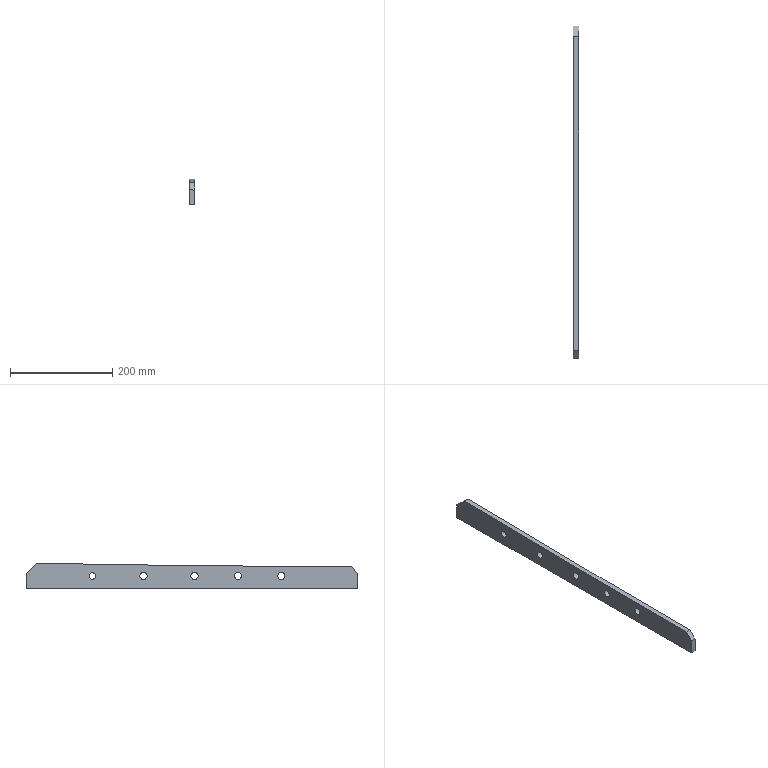Part | NX | features solid 2 | 1 solid | 13 faces | box 10 x 650.034 x 49.781 mm | volume 286400 mm3 | plane 5 | cylinder 5 | spline 3 | commonest cylinder face diameters 14 x4 13 x1
STEP:
#1=CARTESIAN_POINT('',(65.,-179.966,-104.));
#2=VERTEX_POINT('',#1);
#3=CARTESIAN_POINT('',(65.,-179.966,-97.));
#4=DIRECTION('',(1.,0.,0.));
#5=DIRECTION('',(0.,0.,-1.));
#6=AXIS2_PLACEMENT_3D('',#3,#4,#5);
#7=CIRCLE('',#6,7.);
#8=EDGE_CURVE('',#2,#2,#7,.F.);
#9=ORIENTED_EDGE('',*,*,#8,.T.);
#10=EDGE_LOOP('',(#9));
#11=FACE_BOUND('',#10,.T.);
#12=CARTESIAN_POINT('',(65.,-9.966,-104.));
#13=VERTEX_POINT('',#12);
#14=CARTESIAN_POINT('',(65.,-9.966,-97.));
#15=DIRECTION('',(1.,0.,0.));
#16=DIRECTION('',(0.,0.,-1.));
#17=AXIS2_PLACEMENT_3D('',#14,#15,#16);
#18=CIRCLE('',#17,7.);
#19=EDGE_CURVE('',#13,#13,#18,.F.);
#20=ORIENTED_EDGE('',*,*,#19,.T.);
#21=EDGE_LOOP('',(#20));
#22=FACE_BOUND('',#21,.T.);
#23=CARTESIAN_POINT('',(65.,190.034,-103.5));
#24=VERTEX_POINT('',#23);
#25=CARTESIAN_POINT('',(65.,190.034,-97.));
#26=DIRECTION('',(1.,0.,0.));
#27=DIRECTION('',(0.,0.,-1.));
#28=AXIS2_PLACEMENT_3D('',#25,#26,#27);
#29=CIRCLE('',#28,6.5);
#30=EDGE_CURVE('',#24,#24,#29,.F.);
#31=ORIENTED_EDGE('',*,*,#30,.T.);
#32=EDGE_LOOP('',(#31));
#33=FACE_BOUND('',#32,.T.);
#34=CARTESIAN_POINT('',(65.,-315.018,-78.578));
#35=VERTEX_POINT('',#34);
#36=CARTESIAN_POINT('',(65.,298.8,-72.24));
#37=VERTEX_POINT('',#36);
#38=CARTESIAN_POINT('',(65.,-315.018,-78.578));
#39=CARTESIAN_POINT('',(65.,-263.862,-78.546));
#40=CARTESIAN_POINT('',(65.,-161.552,-78.297));
#41=CARTESIAN_POINT('',(65.,-33.668,-77.357));
#42=CARTESIAN_POINT('',(65.,68.633,-76.074));
#43=CARTESIAN_POINT('',(65.,170.929,-74.342));
#44=CARTESIAN_POINT('',(65.,247.652,-73.087));
#45=CARTESIAN_POINT('',(65.,298.8,-72.24));
#46=B_SPLINE_CURVE_WITH_KNOTS('',3,(#38,#39,#40,#41,#42,#43,#44,#45),.UNSPECIFIED.,.F.,.F.,(4,1,1,1,1,4),(0.,0.1535,0.3069,0.3837,0.4604,0.6139),.UNSPECIFIED.);
#47=EDGE_CURVE('',#35,#37,#46,.T.);
#48=ORIENTED_EDGE('',*,*,#47,.F.);
#49=CARTESIAN_POINT('',(65.,-330.,-93.701));
#50=VERTEX_POINT('',#49);
#51=CARTESIAN_POINT('',(65.,-315.018,-78.578));
#52=CARTESIAN_POINT('',(65.,-320.012,-83.619));
#53=CARTESIAN_POINT('',(65.,-325.006,-88.66));
#54=CARTESIAN_POINT('',(65.,-330.,-93.701));
#55=B_SPLINE_CURVE_WITH_KNOTS('',3,(#51,#52,#53,#54),.UNSPECIFIED.,.F.,.F.,(4,4),(0.,1.),.UNSPECIFIED.);
#56=EDGE_CURVE('',#35,#50,#55,.T.);
#57=ORIENTED_EDGE('',*,*,#56,.T.);
#58=CARTESIAN_POINT('',(65.,-330.,-122.));
#59=VERTEX_POINT('',#58);
#60=CARTESIAN_POINT('',(65.,-330.,-89.38));
#61=DIRECTION('',(0.,0.,-1.));
#62=VECTOR('',#61,1000.);
#63=LINE('',#60,#62);
#64=EDGE_CURVE('',#59,#50,#63,.F.);
#65=ORIENTED_EDGE('',*,*,#64,.F.);
#66=CARTESIAN_POINT('',(65.,320.034,-122.));
#67=VERTEX_POINT('',#66);
#68=CARTESIAN_POINT('',(65.,-238.872,-122.));
#69=DIRECTION('',(0.,1.,0.));
#70=VECTOR('',#69,1000.);
#71=LINE('',#68,#70);
#72=EDGE_CURVE('',#59,#67,#71,.T.);
#73=ORIENTED_EDGE('',*,*,#72,.T.);
#74=CARTESIAN_POINT('',(65.,320.034,-93.301));
#75=VERTEX_POINT('',#74);
#76=CARTESIAN_POINT('',(65.,320.034,-89.38));
#77=DIRECTION('',(0.,0.,-1.));
#78=VECTOR('',#77,1000.);
#79=LINE('',#76,#78);
#80=EDGE_CURVE('',#75,#67,#79,.T.);
#81=ORIENTED_EDGE('',*,*,#80,.F.);
#82=CARTESIAN_POINT('',(65.,298.8,-72.24));
#83=CARTESIAN_POINT('',(65.,305.878,-79.261));
#84=CARTESIAN_POINT('',(65.,312.956,-86.281));
#85=CARTESIAN_POINT('',(65.,320.034,-93.301));
#86=B_SPLINE_CURVE_WITH_KNOTS('',3,(#82,#83,#84,#85),.UNSPECIFIED.,.F.,.F.,(4,4),(-0.002311,0.0276),.UNSPECIFIED.);
#87=EDGE_CURVE('',#37,#75,#86,.T.);
#88=ORIENTED_EDGE('',*,*,#87,.F.);
#89=EDGE_LOOP('',(#48,#57,#65,#73,#81,#88));
#90=FACE_BOUND('',#89,.T.);
#91=CARTESIAN_POINT('',(65.,90.034,-104.));
#92=VERTEX_POINT('',#91);
#93=CARTESIAN_POINT('',(65.,90.034,-97.));
#94=DIRECTION('',(1.,0.,0.));
#95=DIRECTION('',(0.,0.,-1.));
#96=AXIS2_PLACEMENT_3D('',#93,#94,#95);
#97=CIRCLE('',#96,7.);
#98=EDGE_CURVE('',#92,#92,#97,.F.);
#99=ORIENTED_EDGE('',*,*,#98,.T.);
#100=EDGE_LOOP('',(#99));
#101=FACE_BOUND('',#100,.T.);
#102=CARTESIAN_POINT('',(65.,-94.966,-104.));
#103=VERTEX_POINT('',#102);
#104=CARTESIAN_POINT('',(65.,-94.966,-97.));
#105=DIRECTION('',(1.,0.,0.));
#106=DIRECTION('',(0.,0.,-1.));
#107=AXIS2_PLACEMENT_3D('',#104,#105,#106);
#108=CIRCLE('',#107,7.);
#109=EDGE_CURVE('',#103,#103,#108,.F.);
#110=ORIENTED_EDGE('',*,*,#109,.T.);
#111=EDGE_LOOP('',(#110));
#112=FACE_BOUND('',#111,.T.);
#113=CARTESIAN_POINT('',(65.,5.001,-89.38));
#114=DIRECTION('',(-1.,0.,0.));
#115=DIRECTION('',(0.,0.,1.));
#116=AXIS2_PLACEMENT_3D('',#113,#114,#115);
#117=PLANE('',#116);
#118=ADVANCED_FACE('',(#11,#22,#33,#90,#101,#112),#117,.F.);
#119=CARTESIAN_POINT('',(55.,-179.966,-104.));
#120=VERTEX_POINT('',#119);
#121=CARTESIAN_POINT('',(55.,-179.966,-97.));
#122=DIRECTION('',(1.,0.,0.));
#123=DIRECTION('',(0.,0.,-1.));
#124=AXIS2_PLACEMENT_3D('',#121,#122,#123);
#125=CIRCLE('',#124,7.);
#126=EDGE_CURVE('',#120,#120,#125,.T.);
#127=ORIENTED_EDGE('',*,*,#126,.T.);
#128=EDGE_LOOP('',(#127));
#129=FACE_BOUND('',#128,.T.);
#130=CARTESIAN_POINT('',(55.,-9.966,-104.));
#131=VERTEX_POINT('',#130);
#132=CARTESIAN_POINT('',(55.,-9.966,-97.));
#133=DIRECTION('',(1.,0.,0.));
#134=DIRECTION('',(0.,0.,-1.));
#135=AXIS2_PLACEMENT_3D('',#132,#133,#134);
#136=CIRCLE('',#135,7.);
#137=EDGE_CURVE('',#131,#131,#136,.T.);
#138=ORIENTED_EDGE('',*,*,#137,.T.);
#139=EDGE_LOOP('',(#138));
#140=FACE_BOUND('',#139,.T.);
#141=CARTESIAN_POINT('',(55.,190.034,-103.5));
#142=VERTEX_POINT('',#141);
#143=CARTESIAN_POINT('',(55.,190.034,-97.));
#144=DIRECTION('',(1.,0.,0.));
#145=DIRECTION('',(0.,0.,-1.));
#146=AXIS2_PLACEMENT_3D('',#143,#144,#145);
#147=CIRCLE('',#146,6.5);
#148=EDGE_CURVE('',#142,#142,#147,.T.);
#149=ORIENTED_EDGE('',*,*,#148,.T.);
#150=EDGE_LOOP('',(#149));
#151=FACE_BOUND('',#150,.T.);
#152=CARTESIAN_POINT('',(55.,-330.,-122.));
#153=VERTEX_POINT('',#152);
#154=CARTESIAN_POINT('',(55.,-330.,-92.375));
#155=VERTEX_POINT('',#154);
#156=CARTESIAN_POINT('',(55.,-330.,-85.181));
#157=DIRECTION('',(0.,0.,-1.));
#158=VECTOR('',#157,1000.);
#159=LINE('',#156,#158);
#160=EDGE_CURVE('',#153,#155,#159,.F.);
#161=ORIENTED_EDGE('',*,*,#160,.T.);
#162=CARTESIAN_POINT('',(55.,-316.344,-78.579));
#163=VERTEX_POINT('',#162);
#164=CARTESIAN_POINT('',(55.,-330.,-92.375));
#165=CARTESIAN_POINT('',(55.,-325.448,-87.776));
#166=CARTESIAN_POINT('',(55.,-320.896,-83.178));
#167=CARTESIAN_POINT('',(55.,-316.344,-78.579));
#168=B_SPLINE_CURVE_WITH_KNOTS('',3,(#164,#165,#166,#167),.UNSPECIFIED.,.F.,.F.,(4,4),(0.,1.),.UNSPECIFIED.);
#169=EDGE_CURVE('',#155,#163,#168,.T.);
#170=ORIENTED_EDGE('',*,*,#169,.T.);
#171=CARTESIAN_POINT('',(55.,300.081,-72.219));
#172=VERTEX_POINT('',#171);
#173=CARTESIAN_POINT('',(55.,-316.344,-78.579));
#174=CARTESIAN_POINT('',(55.,-264.972,-78.546));
#175=CARTESIAN_POINT('',(55.,-162.227,-78.301));
#176=CARTESIAN_POINT('',(55.,-33.799,-77.359));
#177=CARTESIAN_POINT('',(55.,68.937,-76.07));
#178=CARTESIAN_POINT('',(55.,171.667,-74.329));
#179=CARTESIAN_POINT('',(55.,248.716,-73.069));
#180=CARTESIAN_POINT('',(55.,300.081,-72.219));
#181=B_SPLINE_CURVE_WITH_KNOTS('',3,(#173,#174,#175,#176,#177,#178,#179,#180),.UNSPECIFIED.,.F.,.F.,(4,1,1,1,1,4),(0.,0.1541,0.3082,0.3853,0.4624,0.6165),.UNSPECIFIED.);
#182=EDGE_CURVE('',#163,#172,#181,.T.);
#183=ORIENTED_EDGE('',*,*,#182,.T.);
#184=CARTESIAN_POINT('',(55.,320.034,-92.026));
#185=VERTEX_POINT('',#184);
#186=CARTESIAN_POINT('',(55.,320.034,-92.026));
#187=CARTESIAN_POINT('',(55.,313.383,-85.424));
#188=CARTESIAN_POINT('',(55.,306.732,-78.822));
#189=CARTESIAN_POINT('',(55.,300.081,-72.219));
#190=B_SPLINE_CURVE_WITH_KNOTS('',3,(#186,#187,#188,#189),.UNSPECIFIED.,.F.,.F.,(4,4),(0.,0.02812),.UNSPECIFIED.);
#191=EDGE_CURVE('',#185,#172,#190,.T.);
#192=ORIENTED_EDGE('',*,*,#191,.F.);
#193=CARTESIAN_POINT('',(55.,320.034,-122.));
#194=VERTEX_POINT('',#193);
#195=CARTESIAN_POINT('',(55.,320.034,-85.181));
#196=DIRECTION('',(0.,0.,-1.));
#197=VECTOR('',#196,1000.);
#198=LINE('',#195,#197);
#199=EDGE_CURVE('',#185,#194,#198,.T.);
#200=ORIENTED_EDGE('',*,*,#199,.T.);
#201=CARTESIAN_POINT('',(55.,-238.872,-122.));
#202=DIRECTION('',(0.,1.,0.));
#203=VECTOR('',#202,1000.);
#204=LINE('',#201,#203);
#205=EDGE_CURVE('',#153,#194,#204,.T.);
#206=ORIENTED_EDGE('',*,*,#205,.F.);
#207=EDGE_LOOP('',(#161,#170,#183,#192,#200,#206));
#208=FACE_BOUND('',#207,.T.);
#209=CARTESIAN_POINT('',(55.,90.034,-104.));
#210=VERTEX_POINT('',#209);
#211=CARTESIAN_POINT('',(55.,90.034,-97.));
#212=DIRECTION('',(1.,0.,0.));
#213=DIRECTION('',(0.,0.,-1.));
#214=AXIS2_PLACEMENT_3D('',#211,#212,#213);
#215=CIRCLE('',#214,7.);
#216=EDGE_CURVE('',#210,#210,#215,.T.);
#217=ORIENTED_EDGE('',*,*,#216,.T.);
#218=EDGE_LOOP('',(#217));
#219=FACE_BOUND('',#218,.T.);
#220=CARTESIAN_POINT('',(55.,-94.966,-104.));
#221=VERTEX_POINT('',#220);
#222=CARTESIAN_POINT('',(55.,-94.966,-97.));
#223=DIRECTION('',(1.,0.,0.));
#224=DIRECTION('',(0.,0.,-1.));
#225=AXIS2_PLACEMENT_3D('',#222,#223,#224);
#226=CIRCLE('',#225,7.);
#227=EDGE_CURVE('',#221,#221,#226,.T.);
#228=ORIENTED_EDGE('',*,*,#227,.T.);
#229=EDGE_LOOP('',(#228));
#230=FACE_BOUND('',#229,.T.);
#231=CARTESIAN_POINT('',(55.,5.001,-85.181));
#232=DIRECTION('',(-1.,0.,0.));
#233=DIRECTION('',(0.,0.,1.));
#234=AXIS2_PLACEMENT_3D('',#231,#232,#233);
#235=PLANE('',#234);
#236=ADVANCED_FACE('',(#129,#140,#151,#208,#219,#230),#235,.T.);
#237=ORIENTED_EDGE('',*,*,#148,.F.);
#238=EDGE_LOOP('',(#237));
#239=FACE_BOUND('',#238,.T.);
#240=ORIENTED_EDGE('',*,*,#30,.F.);
#241=EDGE_LOOP('',(#240));
#242=FACE_BOUND('',#241,.T.);
#243=CARTESIAN_POINT('',(85.,190.034,-97.));
#244=DIRECTION('',(-1.,0.,0.));
#245=DIRECTION('',(0.,0.,1.));
#246=AXIS2_PLACEMENT_3D('',#243,#244,#245);
#247=CYLINDRICAL_SURFACE('',#246,6.5);
#248=ADVANCED_FACE('',(#239,#242),#247,.F.);
#249=ORIENTED_EDGE('',*,*,#72,.F.);
#250=CARTESIAN_POINT('',(1013.409,-330.,-122.));
#251=DIRECTION('',(1.,0.,0.));
#252=VECTOR('',#251,1000.);
#253=LINE('',#250,#252);
#254=EDGE_CURVE('',#59,#153,#253,.F.);
#255=ORIENTED_EDGE('',*,*,#254,.T.);
#256=ORIENTED_EDGE('',*,*,#205,.T.);
#257=CARTESIAN_POINT('',(1013.409,320.034,-122.));
#258=DIRECTION('',(1.,0.,0.));
#259=VECTOR('',#258,1000.);
#260=LINE('',#257,#259);
#261=EDGE_CURVE('',#194,#67,#260,.T.);
#262=ORIENTED_EDGE('',*,*,#261,.T.);
#263=EDGE_LOOP('',(#249,#255,#256,#262));
#264=FACE_BOUND('',#263,.T.);
#265=CARTESIAN_POINT('',(1013.409,-238.872,-122.));
#266=DIRECTION('',(0.,0.,-1.));
#267=DIRECTION('',(-1.,0.,0.));
#268=AXIS2_PLACEMENT_3D('',#265,#266,#267);
#269=PLANE('',#268);
#270=ADVANCED_FACE('',(#264),#269,.T.);
#271=ORIENTED_EDGE('',*,*,#80,.T.);
#272=ORIENTED_EDGE('',*,*,#261,.F.);
#273=ORIENTED_EDGE('',*,*,#199,.F.);
#274=CARTESIAN_POINT('',(65.,320.034,-93.301));
#275=CARTESIAN_POINT('',(61.666,320.034,-92.885));
#276=CARTESIAN_POINT('',(58.332,320.034,-92.46));
#277=CARTESIAN_POINT('',(55.,320.034,-92.026));
#278=B_SPLINE_CURVE_WITH_KNOTS('',3,(#274,#275,#276,#277),.UNSPECIFIED.,.F.,.F.,(4,4),(0.,0.01008),.UNSPECIFIED.);
#279=EDGE_CURVE('',#75,#185,#278,.T.);
#280=ORIENTED_EDGE('',*,*,#279,.F.);
#281=EDGE_LOOP('',(#271,#272,#273,#280));
#282=FACE_BOUND('',#281,.T.);
#283=CARTESIAN_POINT('',(395.5,320.034,-62.002));
#284=DIRECTION('',(0.,1.,0.));
#285=DIRECTION('',(0.,0.,1.));
#286=AXIS2_PLACEMENT_3D('',#283,#284,#285);
#287=PLANE('',#286);
#288=ADVANCED_FACE('',(#282),#287,.T.);
#289=ORIENTED_EDGE('',*,*,#182,.F.);
#290=CARTESIAN_POINT('',(55.,-316.344,-78.579));
#291=CARTESIAN_POINT('',(58.332,-315.891,-78.579));
#292=CARTESIAN_POINT('',(61.665,-315.449,-78.578));
#293=CARTESIAN_POINT('',(65.,-315.018,-78.578));
#294=B_SPLINE_CURVE_WITH_KNOTS('',3,(#290,#291,#292,#293),.UNSPECIFIED.,.F.,.F.,(4,4),(0.,0.01009),.UNSPECIFIED.);
#295=EDGE_CURVE('',#163,#35,#294,.T.);
#296=ORIENTED_EDGE('',*,*,#295,.T.);
#297=ORIENTED_EDGE('',*,*,#47,.T.);
#298=CARTESIAN_POINT('',(55.,300.081,-72.219));
#299=CARTESIAN_POINT('',(58.332,299.646,-72.226));
#300=CARTESIAN_POINT('',(61.666,299.219,-72.233));
#301=CARTESIAN_POINT('',(65.,298.8,-72.24));
#302=B_SPLINE_CURVE_WITH_KNOTS('',3,(#298,#299,#300,#301),.UNSPECIFIED.,.F.,.F.,(4,4),(0.,0.01008),.UNSPECIFIED.);
#303=EDGE_CURVE('',#172,#37,#302,.T.);
#304=ORIENTED_EDGE('',*,*,#303,.F.);
#305=EDGE_LOOP('',(#289,#296,#297,#304));
#306=FACE_BOUND('',#305,.T.);
#307=CARTESIAN_POINT('',(65.,-319.189,-78.581));
#308=CARTESIAN_POINT('',(54.94,-319.189,-78.581));
#309=CARTESIAN_POINT('',(65.,-267.271,-78.548));
#310=CARTESIAN_POINT('',(54.94,-267.271,-78.548));
#311=CARTESIAN_POINT('',(65.,-163.437,-78.311));
#312=CARTESIAN_POINT('',(54.94,-163.437,-78.311));
#313=CARTESIAN_POINT('',(65.,-33.646,-77.36));
#314=CARTESIAN_POINT('',(54.94,-33.646,-77.36));
#315=CARTESIAN_POINT('',(65.,70.181,-76.052));
#316=CARTESIAN_POINT('',(54.94,70.181,-76.052));
#317=CARTESIAN_POINT('',(65.,174.002,-74.289));
#318=CARTESIAN_POINT('',(54.94,174.002,-74.289));
#319=CARTESIAN_POINT('',(65.,251.869,-73.017));
#320=CARTESIAN_POINT('',(54.94,251.869,-73.017));
#321=CARTESIAN_POINT('',(65.,303.779,-72.158));
#322=CARTESIAN_POINT('',(54.94,303.779,-72.158));
#323=B_SPLINE_SURFACE_WITH_KNOTS('',3,1,((#307,#308),(#309,#310),(#311,#312),(#313,#314),(#315,#316),(#317,#318),(#319,#320),(#321,#322)),.SURF_OF_LINEAR_EXTRUSION.,.F.,.F.,.F.,(4,1,1,1,1,4),(2,2),(-0.01,0.3634,0.7368,0.9235,1.11,1.484),(0.,1.),.UNSPECIFIED.);
#324=ADVANCED_FACE('',(#306),#323,.T.);
#325=ORIENTED_EDGE('',*,*,#216,.F.);
#326=EDGE_LOOP('',(#325));
#327=FACE_BOUND('',#326,.T.);
#328=ORIENTED_EDGE('',*,*,#98,.F.);
#329=EDGE_LOOP('',(#328));
#330=FACE_BOUND('',#329,.T.);
#331=CARTESIAN_POINT('',(85.,90.034,-97.));
#332=DIRECTION('',(-1.,0.,0.));
#333=DIRECTION('',(0.,0.,1.));
#334=AXIS2_PLACEMENT_3D('',#331,#332,#333);
#335=CYLINDRICAL_SURFACE('',#334,7.);
#336=ADVANCED_FACE('',(#327,#330),#335,.F.);
#337=ORIENTED_EDGE('',*,*,#137,.F.);
#338=EDGE_LOOP('',(#337));
#339=FACE_BOUND('',#338,.T.);
#340=ORIENTED_EDGE('',*,*,#19,.F.);
#341=EDGE_LOOP('',(#340));
#342=FACE_BOUND('',#341,.T.);
#343=CARTESIAN_POINT('',(85.,-9.966,-97.));
#344=DIRECTION('',(-1.,0.,0.));
#345=DIRECTION('',(0.,0.,1.));
#346=AXIS2_PLACEMENT_3D('',#343,#344,#345);
#347=CYLINDRICAL_SURFACE('',#346,7.);
#348=ADVANCED_FACE('',(#339,#342),#347,.F.);
#349=ORIENTED_EDGE('',*,*,#227,.F.);
#350=EDGE_LOOP('',(#349));
#351=FACE_BOUND('',#350,.T.);
#352=ORIENTED_EDGE('',*,*,#109,.F.);
#353=EDGE_LOOP('',(#352));
#354=FACE_BOUND('',#353,.T.);
#355=CARTESIAN_POINT('',(85.,-94.966,-97.));
#356=DIRECTION('',(-1.,0.,0.));
#357=DIRECTION('',(0.,0.,1.));
#358=AXIS2_PLACEMENT_3D('',#355,#356,#357);
#359=CYLINDRICAL_SURFACE('',#358,7.);
#360=ADVANCED_FACE('',(#351,#354),#359,.F.);
#361=ORIENTED_EDGE('',*,*,#126,.F.);
#362=EDGE_LOOP('',(#361));
#363=FACE_BOUND('',#362,.T.);
#364=ORIENTED_EDGE('',*,*,#8,.F.);
#365=EDGE_LOOP('',(#364));
#366=FACE_BOUND('',#365,.T.);
#367=CARTESIAN_POINT('',(85.,-179.966,-97.));
#368=DIRECTION('',(-1.,0.,0.));
#369=DIRECTION('',(0.,0.,1.));
#370=AXIS2_PLACEMENT_3D('',#367,#368,#369);
#371=CYLINDRICAL_SURFACE('',#370,7.);
#372=ADVANCED_FACE('',(#363,#366),#371,.F.);
#373=ORIENTED_EDGE('',*,*,#64,.T.);
#374=CARTESIAN_POINT('',(55.,-330.,-92.375));
#375=CARTESIAN_POINT('',(58.333,-330.,-92.817));
#376=CARTESIAN_POINT('',(61.667,-330.,-93.259));
#377=CARTESIAN_POINT('',(65.,-330.,-93.701));
#378=B_SPLINE_CURVE_WITH_KNOTS('',3,(#374,#375,#376,#377),.UNSPECIFIED.,.F.,.F.,(4,4),(0.,1.),.UNSPECIFIED.);
#379=EDGE_CURVE('',#50,#155,#378,.F.);
#380=ORIENTED_EDGE('',*,*,#379,.T.);
#381=ORIENTED_EDGE('',*,*,#160,.F.);
#382=ORIENTED_EDGE('',*,*,#254,.F.);
#383=EDGE_LOOP('',(#373,#380,#381,#382));
#384=FACE_BOUND('',#383,.T.);
#385=CARTESIAN_POINT('',(140.,-330.,-176.968));
#386=DIRECTION('',(0.,1.,0.));
#387=DIRECTION('',(0.,0.,1.));
#388=AXIS2_PLACEMENT_3D('',#385,#386,#387);
#389=PLANE('',#388);
#390=ADVANCED_FACE('',(#384),#389,.F.);
#391=ORIENTED_EDGE('',*,*,#191,.T.);
#392=ORIENTED_EDGE('',*,*,#303,.T.);
#393=ORIENTED_EDGE('',*,*,#87,.T.);
#394=ORIENTED_EDGE('',*,*,#279,.T.);
#395=EDGE_LOOP('',(#391,#392,#393,#394));
#396=FACE_BOUND('',#395,.T.);
#397=CARTESIAN_POINT('',(55.106,298.678,-70.84));
#398=CARTESIAN_POINT('',(59.296,298.675,-71.39));
#399=CARTESIAN_POINT('',(63.487,298.673,-71.927));
#400=CARTESIAN_POINT('',(67.676,298.672,-72.449));
#401=CARTESIAN_POINT('',(54.186,305.84,-77.829));
#402=CARTESIAN_POINT('',(58.392,305.838,-78.381));
#403=CARTESIAN_POINT('',(62.598,305.836,-78.92));
#404=CARTESIAN_POINT('',(66.804,305.835,-79.444));
#405=CARTESIAN_POINT('',(53.267,313.001,-84.818));
#406=CARTESIAN_POINT('',(57.488,313.,-85.372));
#407=CARTESIAN_POINT('',(61.71,312.999,-85.913));
#408=CARTESIAN_POINT('',(65.932,312.998,-86.439));
#409=CARTESIAN_POINT('',(52.348,320.163,-91.807));
#410=CARTESIAN_POINT('',(56.584,320.162,-92.363));
#411=CARTESIAN_POINT('',(60.822,320.162,-92.906));
#412=CARTESIAN_POINT('',(65.06,320.162,-93.434));
#413=B_SPLINE_SURFACE_WITH_KNOTS('',3,3,((#397,#398,#399,#400),(#401,#402,#403,#404),(#405,#406,#407,#408),(#409,#410,#411,#412)),.UNSPECIFIED.,.F.,.F.,.F.,(4,4),(4,4),(0.003847,0.8646),(0.09403,0.1069),.UNSPECIFIED.);
#414=ADVANCED_FACE('',(#396),#413,.F.);
#415=ORIENTED_EDGE('',*,*,#56,.F.);
#416=ORIENTED_EDGE('',*,*,#295,.F.);
#417=ORIENTED_EDGE('',*,*,#169,.F.);
#418=ORIENTED_EDGE('',*,*,#379,.F.);
#419=EDGE_LOOP('',(#415,#416,#417,#418));
#420=FACE_BOUND('',#419,.T.);
#421=CARTESIAN_POINT('',(65.071,-330.,-93.71));
#422=CARTESIAN_POINT('',(61.069,-330.,-93.194));
#423=CARTESIAN_POINT('',(57.068,-330.,-92.66));
#424=CARTESIAN_POINT('',(53.07,-330.,-92.111));
#425=CARTESIAN_POINT('',(66.992,-315.006,-78.824));
#426=CARTESIAN_POINT('',(63.032,-315.005,-78.313));
#427=CARTESIAN_POINT('',(59.071,-315.005,-77.785));
#428=CARTESIAN_POINT('',(55.112,-315.005,-77.241));
#429=B_SPLINE_SURFACE_WITH_KNOTS('',1,3,((#421,#422,#423,#424),(#425,#426,#427,#428)),.RULED_SURF.,.F.,.F.,.F.,(2,2),(4,4),(0.,1.),(0.1468,0.1589),.PIECEWISE_BEZIER_KNOTS.);
#430=ADVANCED_FACE('',(#420),#429,.T.);
#431=CLOSED_SHELL('',(#118,#236,#248,#270,#288,#324,#336,#348,#360,#372,#390,#414,#430));
#432=MANIFOLD_SOLID_BREP('',#431);
#433=(LENGTH_UNIT()NAMED_UNIT(*)SI_UNIT(.MILLI.,.METRE.));
#434=UNCERTAINTY_MEASURE_WITH_UNIT(LENGTH_MEASURE(0.1016),#433,'','');
#435=(NAMED_UNIT(*)PLANE_ANGLE_UNIT()SI_UNIT($,.RADIAN.));
#436=(NAMED_UNIT(*)SI_UNIT($,.STERADIAN.)SOLID_ANGLE_UNIT());
#437=(GEOMETRIC_REPRESENTATION_CONTEXT(3)GLOBAL_UNCERTAINTY_ASSIGNED_CONTEXT((#434))GLOBAL_UNIT_ASSIGNED_CONTEXT((#433,#435,#436))REPRESENTATION_CONTEXT('',''));
#438=ADVANCED_BREP_SHAPE_REPRESENTATION('',(#432),#437);